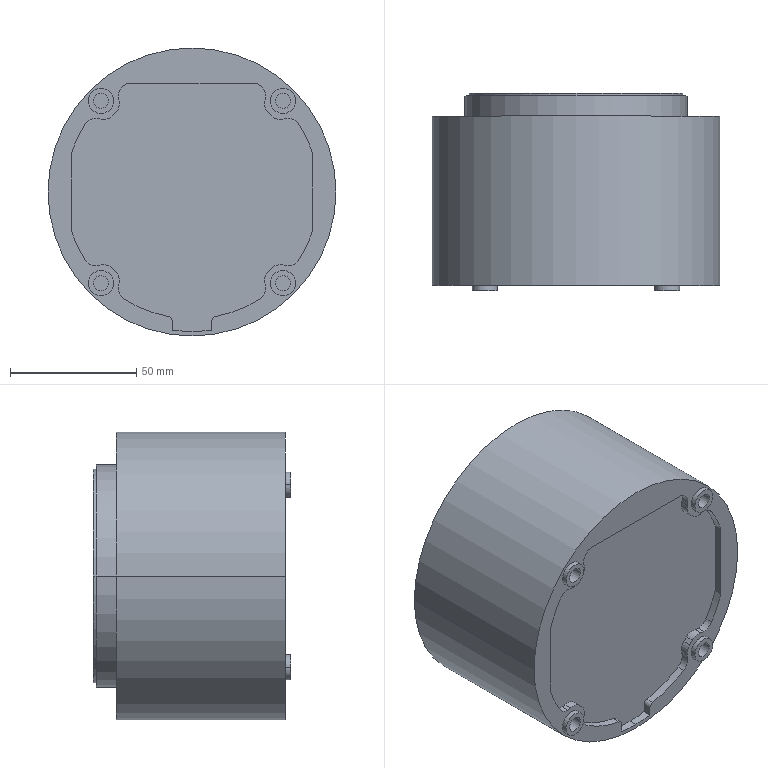Part | NX | features BREP 1 | 1 solid | 122 faces | box 114 x 78 x 114 mm | volume 560505 mm3 | cylinder 84 | plane 26 | cone 12 | commonest cylinder face diameters 3.2 x12 6 x12 10 x8 110 x7 9.748 x5 10.261 x5